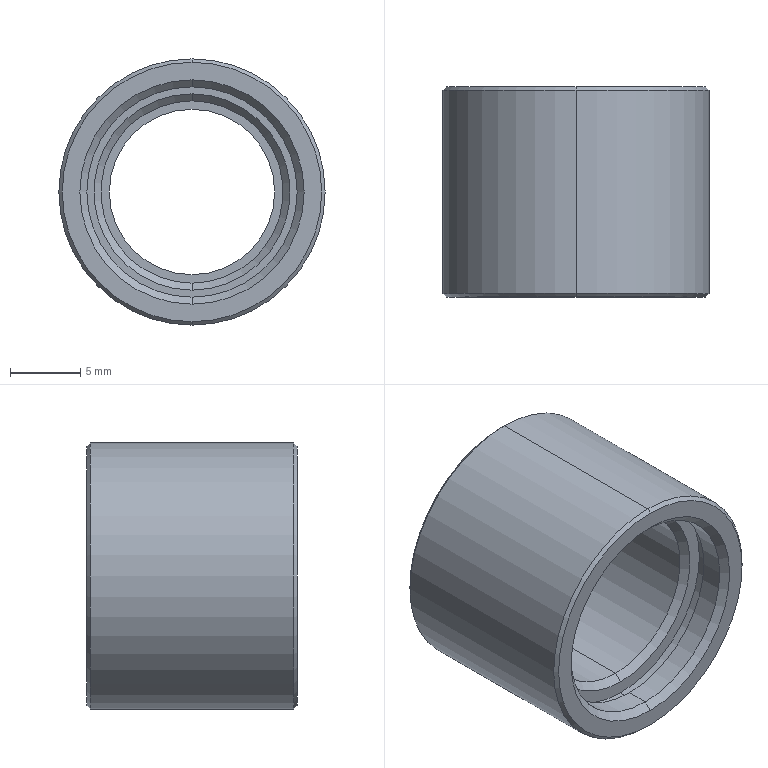Part | NX | features BREP 1 | 1 solid | 25 faces | box 19 x 15 x 19 mm | volume 2137 mm3 | cone 10 | cylinder 10 | plane 5 | commonest cylinder face diameters 11.8 x2 13 x2 15 x2 15.9 x2 19 x2
STEP:
#1=CARTESIAN_POINT('',(0.,0.25,-9.5));
#2=VERTEX_POINT('',#1);
#3=CARTESIAN_POINT('',(0.,0.,-9.25));
#4=VERTEX_POINT('',#3);
#5=CARTESIAN_POINT('',(0.,0.,-9.25));
#6=DIRECTION('',(0.,0.7071,-0.7071));
#7=VECTOR('',#6,1000.);
#8=LINE('',#5,#7);
#9=EDGE_CURVE('',#2,#4,#8,.F.);
#10=ORIENTED_EDGE('',*,*,#9,.T.);
#11=CARTESIAN_POINT('',(0.,0.,9.25));
#12=VERTEX_POINT('',#11);
#13=CARTESIAN_POINT('',(0.,0.,0.));
#14=DIRECTION('',(0.,-1.,0.));
#15=DIRECTION('',(0.,0.,1.));
#16=AXIS2_PLACEMENT_3D('',#13,#14,#15);
#17=CIRCLE('',#16,9.25);
#18=EDGE_CURVE('',#12,#4,#17,.T.);
#19=ORIENTED_EDGE('',*,*,#18,.F.);
#20=CARTESIAN_POINT('',(0.,0.25,9.5));
#21=VERTEX_POINT('',#20);
#22=CARTESIAN_POINT('',(0.,0.,9.25));
#23=DIRECTION('',(0.,0.7071,0.7071));
#24=VECTOR('',#23,1000.);
#25=LINE('',#22,#24);
#26=EDGE_CURVE('',#21,#12,#25,.F.);
#27=ORIENTED_EDGE('',*,*,#26,.F.);
#28=CARTESIAN_POINT('',(0.,0.25,0.));
#29=DIRECTION('',(0.,1.,0.));
#30=DIRECTION('',(0.,0.,1.));
#31=AXIS2_PLACEMENT_3D('',#28,#29,#30);
#32=CIRCLE('',#31,9.5);
#33=EDGE_CURVE('',#2,#21,#32,.T.);
#34=ORIENTED_EDGE('',*,*,#33,.F.);
#35=EDGE_LOOP('',(#10,#19,#27,#34));
#36=FACE_BOUND('',#35,.T.);
#37=CARTESIAN_POINT('',(0.,0.,0.));
#38=DIRECTION('',(0.,1.,0.));
#39=DIRECTION('',(0.,0.,1.));
#40=AXIS2_PLACEMENT_3D('',#37,#38,#39);
#41=CONICAL_SURFACE('',#40,9.25,0.7854);
#42=ADVANCED_FACE('',(#36),#41,.T.);
#43=CARTESIAN_POINT('',(0.,15.,9.25));
#44=VERTEX_POINT('',#43);
#45=CARTESIAN_POINT('',(0.,14.75,9.5));
#46=VERTEX_POINT('',#45);
#47=CARTESIAN_POINT('',(0.,14.75,9.5));
#48=DIRECTION('',(0.,-0.7071,0.7071));
#49=VECTOR('',#48,1000.);
#50=LINE('',#47,#49);
#51=EDGE_CURVE('',#44,#46,#50,.T.);
#52=ORIENTED_EDGE('',*,*,#51,.F.);
#53=CARTESIAN_POINT('',(0.,15.,-9.25));
#54=VERTEX_POINT('',#53);
#55=CARTESIAN_POINT('',(0.,15.,0.));
#56=DIRECTION('',(0.,1.,0.));
#57=DIRECTION('',(0.,0.,-1.));
#58=AXIS2_PLACEMENT_3D('',#55,#56,#57);
#59=CIRCLE('',#58,9.25);
#60=EDGE_CURVE('',#54,#44,#59,.T.);
#61=ORIENTED_EDGE('',*,*,#60,.F.);
#62=CARTESIAN_POINT('',(0.,14.75,-9.5));
#63=VERTEX_POINT('',#62);
#64=CARTESIAN_POINT('',(0.,14.75,-9.5));
#65=DIRECTION('',(0.,-0.7071,-0.7071));
#66=VECTOR('',#65,1000.);
#67=LINE('',#64,#66);
#68=EDGE_CURVE('',#54,#63,#67,.T.);
#69=ORIENTED_EDGE('',*,*,#68,.T.);
#70=CARTESIAN_POINT('',(0.,14.75,0.));
#71=DIRECTION('',(0.,-1.,0.));
#72=DIRECTION('',(0.,0.,-1.));
#73=AXIS2_PLACEMENT_3D('',#70,#71,#72);
#74=CIRCLE('',#73,9.5);
#75=EDGE_CURVE('',#46,#63,#74,.T.);
#76=ORIENTED_EDGE('',*,*,#75,.F.);
#77=EDGE_LOOP('',(#52,#61,#69,#76));
#78=FACE_BOUND('',#77,.T.);
#79=CARTESIAN_POINT('',(0.,14.75,0.));
#80=DIRECTION('',(0.,-1.,0.));
#81=DIRECTION('',(0.,0.,-1.));
#82=AXIS2_PLACEMENT_3D('',#79,#80,#81);
#83=CONICAL_SURFACE('',#82,9.5,0.7854);
#84=ADVANCED_FACE('',(#78),#83,.T.);
#85=CARTESIAN_POINT('',(0.,15.,-6.4));
#86=VERTEX_POINT('',#85);
#87=CARTESIAN_POINT('',(0.,14.5,-5.9));
#88=VERTEX_POINT('',#87);
#89=CARTESIAN_POINT('',(0.,15.,-6.4));
#90=DIRECTION('',(0.,0.7071,-0.7071));
#91=VECTOR('',#90,1000.);
#92=LINE('',#89,#91);
#93=EDGE_CURVE('',#86,#88,#92,.F.);
#94=ORIENTED_EDGE('',*,*,#93,.T.);
#95=CARTESIAN_POINT('',(0.,14.5,5.9));
#96=VERTEX_POINT('',#95);
#97=CARTESIAN_POINT('',(0.,14.5,0.));
#98=DIRECTION('',(0.,1.,0.));
#99=DIRECTION('',(0.,0.,-1.));
#100=AXIS2_PLACEMENT_3D('',#97,#98,#99);
#101=CIRCLE('',#100,5.9);
#102=EDGE_CURVE('',#96,#88,#101,.T.);
#103=ORIENTED_EDGE('',*,*,#102,.F.);
#104=CARTESIAN_POINT('',(0.,15.,6.4));
#105=VERTEX_POINT('',#104);
#106=CARTESIAN_POINT('',(0.,15.,6.4));
#107=DIRECTION('',(0.,0.7071,0.7071));
#108=VECTOR('',#107,1000.);
#109=LINE('',#106,#108);
#110=EDGE_CURVE('',#105,#96,#109,.F.);
#111=ORIENTED_EDGE('',*,*,#110,.F.);
#112=CARTESIAN_POINT('',(0.,15.,0.));
#113=DIRECTION('',(0.,-1.,0.));
#114=DIRECTION('',(0.,0.,-1.));
#115=AXIS2_PLACEMENT_3D('',#112,#113,#114);
#116=CIRCLE('',#115,6.4);
#117=EDGE_CURVE('',#86,#105,#116,.T.);
#118=ORIENTED_EDGE('',*,*,#117,.F.);
#119=EDGE_LOOP('',(#94,#103,#111,#118));
#120=FACE_BOUND('',#119,.T.);
#121=CARTESIAN_POINT('',(0.,15.,0.));
#122=DIRECTION('',(0.,1.,0.));
#123=DIRECTION('',(0.,0.,1.));
#124=AXIS2_PLACEMENT_3D('',#121,#122,#123);
#125=CONICAL_SURFACE('',#124,6.4,0.7854);
#126=ADVANCED_FACE('',(#120),#125,.F.);
#127=CARTESIAN_POINT('',(0.,3.5,6.5));
#128=VERTEX_POINT('',#127);
#129=CARTESIAN_POINT('',(0.,3.,7.));
#130=VERTEX_POINT('',#129);
#131=CARTESIAN_POINT('',(0.,3.5,6.5));
#132=DIRECTION('',(0.,-0.7071,0.7071));
#133=VECTOR('',#132,1000.);
#134=LINE('',#131,#133);
#135=EDGE_CURVE('',#128,#130,#134,.T.);
#136=ORIENTED_EDGE('',*,*,#135,.F.);
#137=CARTESIAN_POINT('',(0.,3.5,-6.5));
#138=VERTEX_POINT('',#137);
#139=CARTESIAN_POINT('',(0.,3.5,0.));
#140=DIRECTION('',(0.,-1.,0.));
#141=DIRECTION('',(0.,0.,1.));
#142=AXIS2_PLACEMENT_3D('',#139,#140,#141);
#143=CIRCLE('',#142,6.5);
#144=EDGE_CURVE('',#138,#128,#143,.T.);
#145=ORIENTED_EDGE('',*,*,#144,.F.);
#146=CARTESIAN_POINT('',(0.,3.,-7.));
#147=VERTEX_POINT('',#146);
#148=CARTESIAN_POINT('',(0.,3.5,-6.5));
#149=DIRECTION('',(0.,-0.7071,-0.7071));
#150=VECTOR('',#149,1000.);
#151=LINE('',#148,#150);
#152=EDGE_CURVE('',#138,#147,#151,.T.);
#153=ORIENTED_EDGE('',*,*,#152,.T.);
#154=CARTESIAN_POINT('',(0.,3.,0.));
#155=DIRECTION('',(0.,1.,0.));
#156=DIRECTION('',(0.,0.,1.));
#157=AXIS2_PLACEMENT_3D('',#154,#155,#156);
#158=CIRCLE('',#157,7.);
#159=EDGE_CURVE('',#130,#147,#158,.T.);
#160=ORIENTED_EDGE('',*,*,#159,.F.);
#161=EDGE_LOOP('',(#136,#145,#153,#160));
#162=FACE_BOUND('',#161,.T.);
#163=CARTESIAN_POINT('',(0.,3.5,0.));
#164=DIRECTION('',(0.,-1.,0.));
#165=DIRECTION('',(0.,0.,-1.));
#166=AXIS2_PLACEMENT_3D('',#163,#164,#165);
#167=CONICAL_SURFACE('',#166,6.5,0.7854);
#168=ADVANCED_FACE('',(#162),#167,.F.);
#169=CARTESIAN_POINT('',(0.,0.5,7.5));
#170=VERTEX_POINT('',#169);
#171=CARTESIAN_POINT('',(0.,0.,8.));
#172=VERTEX_POINT('',#171);
#173=CARTESIAN_POINT('',(0.,0.5,7.5));
#174=DIRECTION('',(0.,-0.7071,0.7071));
#175=VECTOR('',#174,1000.);
#176=LINE('',#173,#175);
#177=EDGE_CURVE('',#170,#172,#176,.T.);
#178=ORIENTED_EDGE('',*,*,#177,.F.);
#179=CARTESIAN_POINT('',(0.,0.5,-7.5));
#180=VERTEX_POINT('',#179);
#181=CARTESIAN_POINT('',(0.,0.5,0.));
#182=DIRECTION('',(0.,-1.,0.));
#183=DIRECTION('',(0.,0.,1.));
#184=AXIS2_PLACEMENT_3D('',#181,#182,#183);
#185=CIRCLE('',#184,7.5);
#186=EDGE_CURVE('',#180,#170,#185,.T.);
#187=ORIENTED_EDGE('',*,*,#186,.F.);
#188=CARTESIAN_POINT('',(0.,0.,-8.));
#189=VERTEX_POINT('',#188);
#190=CARTESIAN_POINT('',(0.,0.5,-7.5));
#191=DIRECTION('',(0.,-0.7071,-0.7071));
#192=VECTOR('',#191,1000.);
#193=LINE('',#190,#192);
#194=EDGE_CURVE('',#180,#189,#193,.T.);
#195=ORIENTED_EDGE('',*,*,#194,.T.);
#196=CARTESIAN_POINT('',(0.,0.,0.));
#197=DIRECTION('',(0.,1.,0.));
#198=DIRECTION('',(0.,0.,1.));
#199=AXIS2_PLACEMENT_3D('',#196,#197,#198);
#200=CIRCLE('',#199,8.);
#201=EDGE_CURVE('',#172,#189,#200,.T.);
#202=ORIENTED_EDGE('',*,*,#201,.F.);
#203=EDGE_LOOP('',(#178,#187,#195,#202));
#204=FACE_BOUND('',#203,.T.);
#205=CARTESIAN_POINT('',(0.,0.5,0.));
#206=DIRECTION('',(0.,-1.,0.));
#207=DIRECTION('',(0.,0.,-1.));
#208=AXIS2_PLACEMENT_3D('',#205,#206,#207);
#209=CONICAL_SURFACE('',#208,7.5,0.7854);
#210=ADVANCED_FACE('',(#204),#209,.F.);
#211=CARTESIAN_POINT('',(0.,2.1,7.5));
#212=VERTEX_POINT('',#211);
#213=CARTESIAN_POINT('',(0.,0.,7.5));
#214=DIRECTION('',(0.,-1.,0.));
#215=VECTOR('',#214,1000.);
#216=LINE('',#213,#215);
#217=EDGE_CURVE('',#212,#170,#216,.T.);
#218=ORIENTED_EDGE('',*,*,#217,.F.);
#219=CARTESIAN_POINT('',(0.,2.1,-7.5));
#220=VERTEX_POINT('',#219);
#221=CARTESIAN_POINT('',(0.,2.1,0.));
#222=DIRECTION('',(0.,-1.,0.));
#223=DIRECTION('',(0.,0.,-1.));
#224=AXIS2_PLACEMENT_3D('',#221,#222,#223);
#225=CIRCLE('',#224,7.5);
#226=EDGE_CURVE('',#220,#212,#225,.T.);
#227=ORIENTED_EDGE('',*,*,#226,.F.);
#228=CARTESIAN_POINT('',(0.,0.,-7.5));
#229=DIRECTION('',(0.,-1.,0.));
#230=VECTOR('',#229,1000.);
#231=LINE('',#228,#230);
#232=EDGE_CURVE('',#220,#180,#231,.T.);
#233=ORIENTED_EDGE('',*,*,#232,.T.);
#234=ORIENTED_EDGE('',*,*,#186,.T.);
#235=EDGE_LOOP('',(#218,#227,#233,#234));
#236=FACE_BOUND('',#235,.T.);
#237=CARTESIAN_POINT('',(0.,0.,0.));
#238=DIRECTION('',(0.,-1.,0.));
#239=DIRECTION('',(0.,0.,-1.));
#240=AXIS2_PLACEMENT_3D('',#237,#238,#239);
#241=CYLINDRICAL_SURFACE('',#240,7.5);
#242=ADVANCED_FACE('',(#236),#241,.F.);
#243=ORIENTED_EDGE('',*,*,#226,.T.);
#244=CARTESIAN_POINT('',(0.,2.1,0.));
#245=DIRECTION('',(0.,-1.,0.));
#246=DIRECTION('',(0.,0.,-1.));
#247=AXIS2_PLACEMENT_3D('',#244,#245,#246);
#248=CIRCLE('',#247,7.5);
#249=EDGE_CURVE('',#212,#220,#248,.T.);
#250=ORIENTED_EDGE('',*,*,#249,.T.);
#251=EDGE_LOOP('',(#243,#250));
#252=FACE_BOUND('',#251,.T.);
#253=CARTESIAN_POINT('',(0.,2.1,-7.95));
#254=VERTEX_POINT('',#253);
#255=CARTESIAN_POINT('',(0.,2.1,7.95));
#256=VERTEX_POINT('',#255);
#257=CARTESIAN_POINT('',(0.,2.1,0.));
#258=DIRECTION('',(0.,-1.,0.));
#259=DIRECTION('',(0.,0.,-1.));
#260=AXIS2_PLACEMENT_3D('',#257,#258,#259);
#261=CIRCLE('',#260,7.95);
#262=EDGE_CURVE('',#254,#256,#261,.T.);
#263=ORIENTED_EDGE('',*,*,#262,.F.);
#264=CARTESIAN_POINT('',(0.,2.1,0.));
#265=DIRECTION('',(0.,-1.,0.));
#266=DIRECTION('',(0.,0.,-1.));
#267=AXIS2_PLACEMENT_3D('',#264,#265,#266);
#268=CIRCLE('',#267,7.95);
#269=EDGE_CURVE('',#256,#254,#268,.T.);
#270=ORIENTED_EDGE('',*,*,#269,.F.);
#271=EDGE_LOOP('',(#263,#270));
#272=FACE_BOUND('',#271,.T.);
#273=CARTESIAN_POINT('',(-7.95,2.1,0.));
#274=DIRECTION('',(0.,-1.,0.));
#275=DIRECTION('',(0.,0.,-1.));
#276=AXIS2_PLACEMENT_3D('',#273,#274,#275);
#277=PLANE('',#276);
#278=ADVANCED_FACE('',(#252,#272),#277,.F.);
#279=CARTESIAN_POINT('',(0.,3.,7.95));
#280=VERTEX_POINT('',#279);
#281=CARTESIAN_POINT('',(0.,0.,7.95));
#282=DIRECTION('',(0.,-1.,0.));
#283=VECTOR('',#282,1000.);
#284=LINE('',#281,#283);
#285=EDGE_CURVE('',#280,#256,#284,.T.);
#286=ORIENTED_EDGE('',*,*,#285,.F.);
#287=CARTESIAN_POINT('',(0.,3.,-7.95));
#288=VERTEX_POINT('',#287);
#289=CARTESIAN_POINT('',(0.,3.,0.));
#290=DIRECTION('',(0.,-1.,0.));
#291=DIRECTION('',(0.,0.,-1.));
#292=AXIS2_PLACEMENT_3D('',#289,#290,#291);
#293=CIRCLE('',#292,7.95);
#294=EDGE_CURVE('',#288,#280,#293,.T.);
#295=ORIENTED_EDGE('',*,*,#294,.F.);
#296=CARTESIAN_POINT('',(0.,0.,-7.95));
#297=DIRECTION('',(0.,-1.,0.));
#298=VECTOR('',#297,1000.);
#299=LINE('',#296,#298);
#300=EDGE_CURVE('',#288,#254,#299,.T.);
#301=ORIENTED_EDGE('',*,*,#300,.T.);
#302=ORIENTED_EDGE('',*,*,#262,.T.);
#303=EDGE_LOOP('',(#286,#295,#301,#302));
#304=FACE_BOUND('',#303,.T.);
#305=CARTESIAN_POINT('',(0.,0.,0.));
#306=DIRECTION('',(0.,-1.,0.));
#307=DIRECTION('',(0.,0.,-1.));
#308=AXIS2_PLACEMENT_3D('',#305,#306,#307);
#309=CYLINDRICAL_SURFACE('',#308,7.95);
#310=ADVANCED_FACE('',(#304),#309,.F.);
#311=ORIENTED_EDGE('',*,*,#294,.T.);
#312=CARTESIAN_POINT('',(0.,3.,0.));
#313=DIRECTION('',(0.,-1.,0.));
#314=DIRECTION('',(0.,0.,-1.));
#315=AXIS2_PLACEMENT_3D('',#312,#313,#314);
#316=CIRCLE('',#315,7.95);
#317=EDGE_CURVE('',#280,#288,#316,.T.);
#318=ORIENTED_EDGE('',*,*,#317,.T.);
#319=EDGE_LOOP('',(#311,#318));
#320=FACE_BOUND('',#319,.T.);
#321=CARTESIAN_POINT('',(0.,3.,0.));
#322=DIRECTION('',(0.,1.,0.));
#323=DIRECTION('',(0.,0.,1.));
#324=AXIS2_PLACEMENT_3D('',#321,#322,#323);
#325=CIRCLE('',#324,7.);
#326=EDGE_CURVE('',#147,#130,#325,.T.);
#327=ORIENTED_EDGE('',*,*,#326,.T.);
#328=ORIENTED_EDGE('',*,*,#159,.T.);
#329=EDGE_LOOP('',(#327,#328));
#330=FACE_BOUND('',#329,.T.);
#331=CARTESIAN_POINT('',(-6.5,3.,0.));
#332=DIRECTION('',(0.,1.,0.));
#333=DIRECTION('',(0.,0.,1.));
#334=AXIS2_PLACEMENT_3D('',#331,#332,#333);
#335=PLANE('',#334);
#336=ADVANCED_FACE('',(#320,#330),#335,.F.);
#337=CARTESIAN_POINT('',(0.,13.,6.5));
#338=VERTEX_POINT('',#337);
#339=CARTESIAN_POINT('',(0.,0.,6.5));
#340=DIRECTION('',(0.,-1.,0.));
#341=VECTOR('',#340,1000.);
#342=LINE('',#339,#341);
#343=EDGE_CURVE('',#338,#128,#342,.T.);
#344=ORIENTED_EDGE('',*,*,#343,.F.);
#345=CARTESIAN_POINT('',(0.,13.,-6.5));
#346=VERTEX_POINT('',#345);
#347=CARTESIAN_POINT('',(0.,13.,0.));
#348=DIRECTION('',(0.,-1.,0.));
#349=DIRECTION('',(0.,0.,-1.));
#350=AXIS2_PLACEMENT_3D('',#347,#348,#349);
#351=CIRCLE('',#350,6.5);
#352=EDGE_CURVE('',#346,#338,#351,.T.);
#353=ORIENTED_EDGE('',*,*,#352,.F.);
#354=CARTESIAN_POINT('',(0.,0.,-6.5));
#355=DIRECTION('',(0.,-1.,0.));
#356=VECTOR('',#355,1000.);
#357=LINE('',#354,#356);
#358=EDGE_CURVE('',#346,#138,#357,.T.);
#359=ORIENTED_EDGE('',*,*,#358,.T.);
#360=ORIENTED_EDGE('',*,*,#144,.T.);
#361=EDGE_LOOP('',(#344,#353,#359,#360));
#362=FACE_BOUND('',#361,.T.);
#363=CARTESIAN_POINT('',(0.,0.,0.));
#364=DIRECTION('',(0.,-1.,0.));
#365=DIRECTION('',(0.,0.,-1.));
#366=AXIS2_PLACEMENT_3D('',#363,#364,#365);
#367=CYLINDRICAL_SURFACE('',#366,6.5);
#368=ADVANCED_FACE('',(#362),#367,.F.);
#369=ORIENTED_EDGE('',*,*,#352,.T.);
#370=CARTESIAN_POINT('',(0.,13.,0.));
#371=DIRECTION('',(0.,-1.,0.));
#372=DIRECTION('',(0.,0.,-1.));
#373=AXIS2_PLACEMENT_3D('',#370,#371,#372);
#374=CIRCLE('',#373,6.5);
#375=EDGE_CURVE('',#338,#346,#374,.T.);
#376=ORIENTED_EDGE('',*,*,#375,.T.);
#377=EDGE_LOOP('',(#369,#376));
#378=FACE_BOUND('',#377,.T.);
#379=CARTESIAN_POINT('',(0.,13.,-5.9));
#380=VERTEX_POINT('',#379);
#381=CARTESIAN_POINT('',(0.,13.,5.9));
#382=VERTEX_POINT('',#381);
#383=CARTESIAN_POINT('',(0.,13.,0.));
#384=DIRECTION('',(0.,-1.,0.));
#385=DIRECTION('',(0.,0.,-1.));
#386=AXIS2_PLACEMENT_3D('',#383,#384,#385);
#387=CIRCLE('',#386,5.9);
#388=EDGE_CURVE('',#380,#382,#387,.T.);
#389=ORIENTED_EDGE('',*,*,#388,.F.);
#390=CARTESIAN_POINT('',(0.,13.,0.));
#391=DIRECTION('',(0.,-1.,0.));
#392=DIRECTION('',(0.,0.,-1.));
#393=AXIS2_PLACEMENT_3D('',#390,#391,#392);
#394=CIRCLE('',#393,5.9);
#395=EDGE_CURVE('',#382,#380,#394,.T.);
#396=ORIENTED_EDGE('',*,*,#395,.F.);
#397=EDGE_LOOP('',(#389,#396));
#398=FACE_BOUND('',#397,.T.);
#399=CARTESIAN_POINT('',(-5.9,13.,0.));
#400=DIRECTION('',(0.,1.,0.));
#401=DIRECTION('',(0.,0.,1.));
#402=AXIS2_PLACEMENT_3D('',#399,#400,#401);
#403=PLANE('',#402);
#404=ADVANCED_FACE('',(#378,#398),#403,.F.);
#405=CARTESIAN_POINT('',(0.,0.,5.9));
#406=DIRECTION('',(0.,-1.,0.));
#407=VECTOR('',#406,1000.);
#408=LINE('',#405,#407);
#409=EDGE_CURVE('',#96,#382,#408,.T.);
#410=ORIENTED_EDGE('',*,*,#409,.F.);
#411=ORIENTED_EDGE('',*,*,#102,.T.);
#412=CARTESIAN_POINT('',(0.,0.,-5.9));
#413=DIRECTION('',(0.,-1.,0.));
#414=VECTOR('',#413,1000.);
#415=LINE('',#412,#414);
#416=EDGE_CURVE('',#88,#380,#415,.T.);
#417=ORIENTED_EDGE('',*,*,#416,.T.);
#418=ORIENTED_EDGE('',*,*,#388,.T.);
#419=EDGE_LOOP('',(#410,#411,#417,#418));
#420=FACE_BOUND('',#419,.T.);
#421=CARTESIAN_POINT('',(0.,0.,0.));
#422=DIRECTION('',(0.,-1.,0.));
#423=DIRECTION('',(0.,0.,-1.));
#424=AXIS2_PLACEMENT_3D('',#421,#422,#423);
#425=CYLINDRICAL_SURFACE('',#424,5.9);
#426=ADVANCED_FACE('',(#420),#425,.F.);
#427=CARTESIAN_POINT('',(0.,15.,0.));
#428=DIRECTION('',(0.,-1.,0.));
#429=DIRECTION('',(0.,0.,-1.));
#430=AXIS2_PLACEMENT_3D('',#427,#428,#429);
#431=CIRCLE('',#430,6.4);
#432=EDGE_CURVE('',#105,#86,#431,.T.);
#433=ORIENTED_EDGE('',*,*,#432,.T.);
#434=ORIENTED_EDGE('',*,*,#117,.T.);
#435=EDGE_LOOP('',(#433,#434));
#436=FACE_BOUND('',#435,.T.);
#437=ORIENTED_EDGE('',*,*,#60,.T.);
#438=CARTESIAN_POINT('',(0.,15.,0.));
#439=DIRECTION('',(0.,1.,0.));
#440=DIRECTION('',(0.,0.,-1.));
#441=AXIS2_PLACEMENT_3D('',#438,#439,#440);
#442=CIRCLE('',#441,9.25);
#443=EDGE_CURVE('',#44,#54,#442,.T.);
#444=ORIENTED_EDGE('',*,*,#443,.T.);
#445=EDGE_LOOP('',(#437,#444));
#446=FACE_BOUND('',#445,.T.);
#447=CARTESIAN_POINT('',(-5.9,15.,0.));
#448=DIRECTION('',(0.,-1.,0.));
#449=DIRECTION('',(0.,0.,-1.));
#450=AXIS2_PLACEMENT_3D('',#447,#448,#449);
#451=PLANE('',#450);
#452=ADVANCED_FACE('',(#436,#446),#451,.F.);
#453=CARTESIAN_POINT('',(0.,0.,9.5));
#454=DIRECTION('',(0.,-1.,0.));
#455=VECTOR('',#454,1000.);
#456=LINE('',#453,#455);
#457=EDGE_CURVE('',#46,#21,#456,.T.);
#458=ORIENTED_EDGE('',*,*,#457,.F.);
#459=ORIENTED_EDGE('',*,*,#75,.T.);
#460=CARTESIAN_POINT('',(0.,0.,-9.5));
#461=DIRECTION('',(0.,-1.,0.));
#462=VECTOR('',#461,1000.);
#463=LINE('',#460,#462);
#464=EDGE_CURVE('',#63,#2,#463,.T.);
#465=ORIENTED_EDGE('',*,*,#464,.T.);
#466=ORIENTED_EDGE('',*,*,#33,.T.);
#467=EDGE_LOOP('',(#458,#459,#465,#466));
#468=FACE_BOUND('',#467,.T.);
#469=CARTESIAN_POINT('',(0.,0.,0.));
#470=DIRECTION('',(0.,-1.,0.));
#471=DIRECTION('',(0.,0.,-1.));
#472=AXIS2_PLACEMENT_3D('',#469,#470,#471);
#473=CYLINDRICAL_SURFACE('',#472,9.5);
#474=ADVANCED_FACE('',(#468),#473,.T.);
#475=CARTESIAN_POINT('',(0.,0.,0.));
#476=DIRECTION('',(0.,1.,0.));
#477=DIRECTION('',(0.,0.,1.));
#478=AXIS2_PLACEMENT_3D('',#475,#476,#477);
#479=CIRCLE('',#478,8.);
#480=EDGE_CURVE('',#189,#172,#479,.T.);
#481=ORIENTED_EDGE('',*,*,#480,.T.);
#482=ORIENTED_EDGE('',*,*,#201,.T.);
#483=EDGE_LOOP('',(#481,#482));
#484=FACE_BOUND('',#483,.T.);
#485=ORIENTED_EDGE('',*,*,#18,.T.);
#486=CARTESIAN_POINT('',(0.,0.,0.));
#487=DIRECTION('',(0.,-1.,0.));
#488=DIRECTION('',(0.,0.,1.));
#489=AXIS2_PLACEMENT_3D('',#486,#487,#488);
#490=CIRCLE('',#489,9.25);
#491=EDGE_CURVE('',#4,#12,#490,.T.);
#492=ORIENTED_EDGE('',*,*,#491,.T.);
#493=EDGE_LOOP('',(#485,#492));
#494=FACE_BOUND('',#493,.T.);
#495=CARTESIAN_POINT('',(-9.5,0.,0.));
#496=DIRECTION('',(0.,1.,0.));
#497=DIRECTION('',(0.,0.,1.));
#498=AXIS2_PLACEMENT_3D('',#495,#496,#497);
#499=PLANE('',#498);
#500=ADVANCED_FACE('',(#484,#494),#499,.F.);
#501=CARTESIAN_POINT('',(0.,14.75,0.));
#502=DIRECTION('',(0.,-1.,0.));
#503=DIRECTION('',(0.,0.,-1.));
#504=AXIS2_PLACEMENT_3D('',#501,#502,#503);
#505=CIRCLE('',#504,9.5);
#506=EDGE_CURVE('',#63,#46,#505,.T.);
#507=ORIENTED_EDGE('',*,*,#506,.T.);
#508=ORIENTED_EDGE('',*,*,#457,.T.);
#509=CARTESIAN_POINT('',(0.,0.25,0.));
#510=DIRECTION('',(0.,1.,0.));
#511=DIRECTION('',(0.,0.,1.));
#512=AXIS2_PLACEMENT_3D('',#509,#510,#511);
#513=CIRCLE('',#512,9.5);
#514=EDGE_CURVE('',#21,#2,#513,.T.);
#515=ORIENTED_EDGE('',*,*,#514,.T.);
#516=ORIENTED_EDGE('',*,*,#464,.F.);
#517=EDGE_LOOP('',(#507,#508,#515,#516));
#518=FACE_BOUND('',#517,.T.);
#519=CARTESIAN_POINT('',(0.,0.,0.));
#520=DIRECTION('',(0.,-1.,0.));
#521=DIRECTION('',(0.,0.,-1.));
#522=AXIS2_PLACEMENT_3D('',#519,#520,#521);
#523=CYLINDRICAL_SURFACE('',#522,9.5);
#524=ADVANCED_FACE('',(#518),#523,.T.);
#525=CARTESIAN_POINT('',(0.,14.5,0.));
#526=DIRECTION('',(0.,1.,0.));
#527=DIRECTION('',(0.,0.,-1.));
#528=AXIS2_PLACEMENT_3D('',#525,#526,#527);
#529=CIRCLE('',#528,5.9);
#530=EDGE_CURVE('',#88,#96,#529,.T.);
#531=ORIENTED_EDGE('',*,*,#530,.T.);
#532=ORIENTED_EDGE('',*,*,#409,.T.);
#533=ORIENTED_EDGE('',*,*,#395,.T.);
#534=ORIENTED_EDGE('',*,*,#416,.F.);
#535=EDGE_LOOP('',(#531,#532,#533,#534));
#536=FACE_BOUND('',#535,.T.);
#537=CARTESIAN_POINT('',(0.,0.,0.));
#538=DIRECTION('',(0.,-1.,0.));
#539=DIRECTION('',(0.,0.,-1.));
#540=AXIS2_PLACEMENT_3D('',#537,#538,#539);
#541=CYLINDRICAL_SURFACE('',#540,5.9);
#542=ADVANCED_FACE('',(#536),#541,.F.);
#543=ORIENTED_EDGE('',*,*,#375,.F.);
#544=ORIENTED_EDGE('',*,*,#343,.T.);
#545=CARTESIAN_POINT('',(0.,3.5,0.));
#546=DIRECTION('',(0.,-1.,0.));
#547=DIRECTION('',(0.,0.,1.));
#548=AXIS2_PLACEMENT_3D('',#545,#546,#547);
#549=CIRCLE('',#548,6.5);
#550=EDGE_CURVE('',#128,#138,#549,.T.);
#551=ORIENTED_EDGE('',*,*,#550,.T.);
#552=ORIENTED_EDGE('',*,*,#358,.F.);
#553=EDGE_LOOP('',(#543,#544,#551,#552));
#554=FACE_BOUND('',#553,.T.);
#555=CARTESIAN_POINT('',(0.,0.,0.));
#556=DIRECTION('',(0.,-1.,0.));
#557=DIRECTION('',(0.,0.,-1.));
#558=AXIS2_PLACEMENT_3D('',#555,#556,#557);
#559=CYLINDRICAL_SURFACE('',#558,6.5);
#560=ADVANCED_FACE('',(#554),#559,.F.);
#561=ORIENTED_EDGE('',*,*,#317,.F.);
#562=ORIENTED_EDGE('',*,*,#285,.T.);
#563=ORIENTED_EDGE('',*,*,#269,.T.);
#564=ORIENTED_EDGE('',*,*,#300,.F.);
#565=EDGE_LOOP('',(#561,#562,#563,#564));
#566=FACE_BOUND('',#565,.T.);
#567=CARTESIAN_POINT('',(0.,0.,0.));
#568=DIRECTION('',(0.,-1.,0.));
#569=DIRECTION('',(0.,0.,-1.));
#570=AXIS2_PLACEMENT_3D('',#567,#568,#569);
#571=CYLINDRICAL_SURFACE('',#570,7.95);
#572=ADVANCED_FACE('',(#566),#571,.F.);
#573=ORIENTED_EDGE('',*,*,#249,.F.);
#574=ORIENTED_EDGE('',*,*,#217,.T.);
#575=CARTESIAN_POINT('',(0.,0.5,0.));
#576=DIRECTION('',(0.,-1.,0.));
#577=DIRECTION('',(0.,0.,1.));
#578=AXIS2_PLACEMENT_3D('',#575,#576,#577);
#579=CIRCLE('',#578,7.5);
#580=EDGE_CURVE('',#170,#180,#579,.T.);
#581=ORIENTED_EDGE('',*,*,#580,.T.);
#582=ORIENTED_EDGE('',*,*,#232,.F.);
#583=EDGE_LOOP('',(#573,#574,#581,#582));
#584=FACE_BOUND('',#583,.T.);
#585=CARTESIAN_POINT('',(0.,0.,0.));
#586=DIRECTION('',(0.,-1.,0.));
#587=DIRECTION('',(0.,0.,-1.));
#588=AXIS2_PLACEMENT_3D('',#585,#586,#587);
#589=CYLINDRICAL_SURFACE('',#588,7.5);
#590=ADVANCED_FACE('',(#584),#589,.F.);
#591=ORIENTED_EDGE('',*,*,#580,.F.);
#592=ORIENTED_EDGE('',*,*,#177,.T.);
#593=ORIENTED_EDGE('',*,*,#480,.F.);
#594=ORIENTED_EDGE('',*,*,#194,.F.);
#595=EDGE_LOOP('',(#591,#592,#593,#594));
#596=FACE_BOUND('',#595,.T.);
#597=CARTESIAN_POINT('',(0.,0.5,0.));
#598=DIRECTION('',(0.,-1.,0.));
#599=DIRECTION('',(0.,0.,-1.));
#600=AXIS2_PLACEMENT_3D('',#597,#598,#599);
#601=CONICAL_SURFACE('',#600,7.5,0.7854);
#602=ADVANCED_FACE('',(#596),#601,.F.);
#603=ORIENTED_EDGE('',*,*,#550,.F.);
#604=ORIENTED_EDGE('',*,*,#135,.T.);
#605=ORIENTED_EDGE('',*,*,#326,.F.);
#606=ORIENTED_EDGE('',*,*,#152,.F.);
#607=EDGE_LOOP('',(#603,#604,#605,#606));
#608=FACE_BOUND('',#607,.T.);
#609=CARTESIAN_POINT('',(0.,3.5,0.));
#610=DIRECTION('',(0.,-1.,0.));
#611=DIRECTION('',(0.,0.,-1.));
#612=AXIS2_PLACEMENT_3D('',#609,#610,#611);
#613=CONICAL_SURFACE('',#612,6.5,0.7854);
#614=ADVANCED_FACE('',(#608),#613,.F.);
#615=ORIENTED_EDGE('',*,*,#530,.F.);
#616=ORIENTED_EDGE('',*,*,#93,.F.);
#617=ORIENTED_EDGE('',*,*,#432,.F.);
#618=ORIENTED_EDGE('',*,*,#110,.T.);
#619=EDGE_LOOP('',(#615,#616,#617,#618));
#620=FACE_BOUND('',#619,.T.);
#621=CARTESIAN_POINT('',(0.,15.,0.));
#622=DIRECTION('',(0.,1.,0.));
#623=DIRECTION('',(0.,0.,1.));
#624=AXIS2_PLACEMENT_3D('',#621,#622,#623);
#625=CONICAL_SURFACE('',#624,6.4,0.7854);
#626=ADVANCED_FACE('',(#620),#625,.F.);
#627=ORIENTED_EDGE('',*,*,#443,.F.);
#628=ORIENTED_EDGE('',*,*,#51,.T.);
#629=ORIENTED_EDGE('',*,*,#506,.F.);
#630=ORIENTED_EDGE('',*,*,#68,.F.);
#631=EDGE_LOOP('',(#627,#628,#629,#630));
#632=FACE_BOUND('',#631,.T.);
#633=CARTESIAN_POINT('',(0.,14.75,0.));
#634=DIRECTION('',(0.,-1.,0.));
#635=DIRECTION('',(0.,0.,-1.));
#636=AXIS2_PLACEMENT_3D('',#633,#634,#635);
#637=CONICAL_SURFACE('',#636,9.5,0.7854);
#638=ADVANCED_FACE('',(#632),#637,.T.);
#639=ORIENTED_EDGE('',*,*,#491,.F.);
#640=ORIENTED_EDGE('',*,*,#9,.F.);
#641=ORIENTED_EDGE('',*,*,#514,.F.);
#642=ORIENTED_EDGE('',*,*,#26,.T.);
#643=EDGE_LOOP('',(#639,#640,#641,#642));
#644=FACE_BOUND('',#643,.T.);
#645=CARTESIAN_POINT('',(0.,0.,0.));
#646=DIRECTION('',(0.,1.,0.));
#647=DIRECTION('',(0.,0.,1.));
#648=AXIS2_PLACEMENT_3D('',#645,#646,#647);
#649=CONICAL_SURFACE('',#648,9.25,0.7854);
#650=ADVANCED_FACE('',(#644),#649,.T.);
#651=CLOSED_SHELL('',(#42,#84,#126,#168,#210,#242,#278,#310,#336,#368,#404,#426,#452,#474,#500,#524,#542,#560,#572,#590,#602,#614,#626,#638,#650));
#652=MANIFOLD_SOLID_BREP('',#651);
#653=(LENGTH_UNIT()NAMED_UNIT(*)SI_UNIT(.MILLI.,.METRE.));
#654=UNCERTAINTY_MEASURE_WITH_UNIT(LENGTH_MEASURE(0.00001),#653,'','');
#655=(NAMED_UNIT(*)PLANE_ANGLE_UNIT()SI_UNIT($,.RADIAN.));
#656=(NAMED_UNIT(*)SI_UNIT($,.STERADIAN.)SOLID_ANGLE_UNIT());
#657=(GEOMETRIC_REPRESENTATION_CONTEXT(3)GLOBAL_UNCERTAINTY_ASSIGNED_CONTEXT((#654))GLOBAL_UNIT_ASSIGNED_CONTEXT((#653,#655,#656))REPRESENTATION_CONTEXT('',''));
#658=ADVANCED_BREP_SHAPE_REPRESENTATION('',(#652),#657);